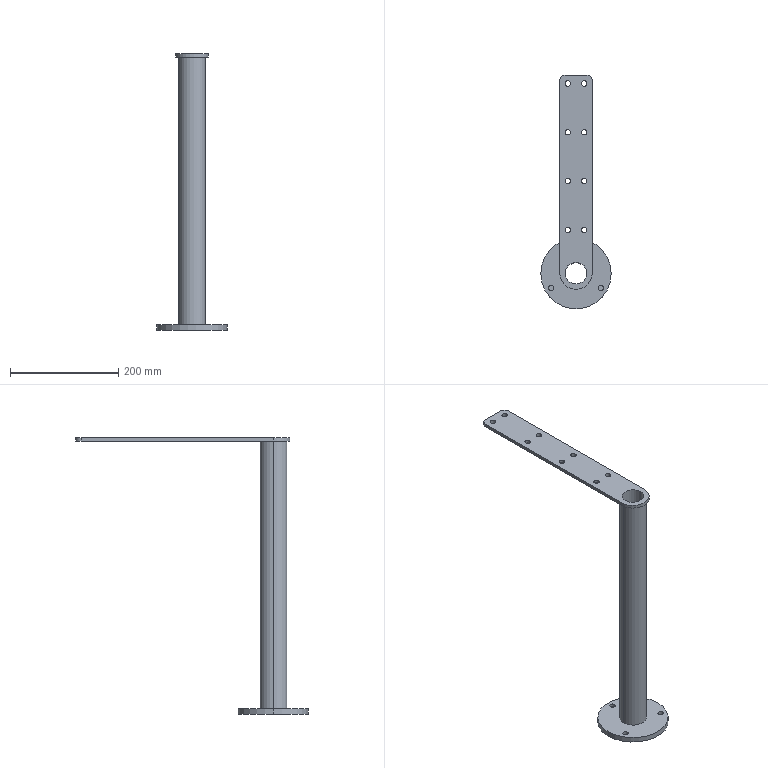Part | SolidWorks | features ICE 4, Extrusion 1, Fillet 1 | 1 solid | 41 faces | box 130 x 430 x 510 mm | volume 596255 mm3 | cylinder 31 | plane 10 | commonest cylinder face diameters 10 x22 20 x2 40 x2 50 x2 130 x2 60 x1
STEP:
#1=CARTESIAN_POINT('',(-5.,53.,4.));
#2=VERTEX_POINT('',#1);
#3=CARTESIAN_POINT('',(5.,53.,4.));
#4=VERTEX_POINT('',#3);
#5=CARTESIAN_POINT('',(0.,53.,4.));
#6=DIRECTION('',(0.,0.,1.));
#7=DIRECTION('',(1.,0.,0.));
#8=AXIS2_PLACEMENT_3D('',#5,#6,#7);
#9=CIRCLE('',#8,5.);
#10=EDGE_CURVE('',#2,#4,#9,.T.);
#11=ORIENTED_EDGE('',*,*,#10,.F.);
#12=CARTESIAN_POINT('',(-5.,53.,10.));
#13=VERTEX_POINT('',#12);
#14=CARTESIAN_POINT('',(-5.,53.,4.));
#15=DIRECTION('',(0.,0.,1.));
#16=VECTOR('',#15,1000.);
#17=LINE('',#14,#16);
#18=EDGE_CURVE('',#2,#13,#17,.T.);
#19=ORIENTED_EDGE('',*,*,#18,.T.);
#20=CARTESIAN_POINT('',(5.,53.,10.));
#21=VERTEX_POINT('',#20);
#22=CARTESIAN_POINT('',(0.,53.,10.));
#23=DIRECTION('',(0.,0.,1.));
#24=DIRECTION('',(1.,0.,0.));
#25=AXIS2_PLACEMENT_3D('',#22,#23,#24);
#26=CIRCLE('',#25,5.);
#27=EDGE_CURVE('',#13,#21,#26,.T.);
#28=ORIENTED_EDGE('',*,*,#27,.T.);
#29=CARTESIAN_POINT('',(5.,53.,4.));
#30=DIRECTION('',(0.,0.,1.));
#31=VECTOR('',#30,1000.);
#32=LINE('',#29,#31);
#33=EDGE_CURVE('',#4,#21,#32,.T.);
#34=ORIENTED_EDGE('',*,*,#33,.F.);
#35=EDGE_LOOP('',(#11,#19,#28,#34));
#36=FACE_OUTER_BOUND('',#35,.T.);
#37=CARTESIAN_POINT('',(0.,53.,4.));
#38=DIRECTION('',(0.,0.,1.));
#39=DIRECTION('',(1.,0.,0.));
#40=AXIS2_PLACEMENT_3D('',#37,#38,#39);
#41=CYLINDRICAL_SURFACE('',#40,5.);
#42=ADVANCED_FACE('',(#36),#41,.F.);
#43=CARTESIAN_POINT('',(40.899,-26.5,4.));
#44=VERTEX_POINT('',#43);
#45=CARTESIAN_POINT('',(50.899,-26.5,4.));
#46=VERTEX_POINT('',#45);
#47=CARTESIAN_POINT('',(45.899,-26.5,4.));
#48=DIRECTION('',(0.,0.,1.));
#49=DIRECTION('',(1.,0.,0.));
#50=AXIS2_PLACEMENT_3D('',#47,#48,#49);
#51=CIRCLE('',#50,5.);
#52=EDGE_CURVE('',#44,#46,#51,.T.);
#53=ORIENTED_EDGE('',*,*,#52,.F.);
#54=CARTESIAN_POINT('',(40.899,-26.5,10.));
#55=VERTEX_POINT('',#54);
#56=CARTESIAN_POINT('',(40.899,-26.5,4.));
#57=DIRECTION('',(0.,0.,1.));
#58=VECTOR('',#57,1000.);
#59=LINE('',#56,#58);
#60=EDGE_CURVE('',#44,#55,#59,.T.);
#61=ORIENTED_EDGE('',*,*,#60,.T.);
#62=CARTESIAN_POINT('',(50.899,-26.5,10.));
#63=VERTEX_POINT('',#62);
#64=CARTESIAN_POINT('',(45.899,-26.5,10.));
#65=DIRECTION('',(0.,0.,1.));
#66=DIRECTION('',(1.,0.,0.));
#67=AXIS2_PLACEMENT_3D('',#64,#65,#66);
#68=CIRCLE('',#67,5.);
#69=EDGE_CURVE('',#55,#63,#68,.T.);
#70=ORIENTED_EDGE('',*,*,#69,.T.);
#71=CARTESIAN_POINT('',(50.899,-26.5,4.));
#72=DIRECTION('',(0.,0.,1.));
#73=VECTOR('',#72,1000.);
#74=LINE('',#71,#73);
#75=EDGE_CURVE('',#46,#63,#74,.T.);
#76=ORIENTED_EDGE('',*,*,#75,.F.);
#77=EDGE_LOOP('',(#53,#61,#70,#76));
#78=FACE_OUTER_BOUND('',#77,.T.);
#79=CARTESIAN_POINT('',(45.899,-26.5,4.));
#80=DIRECTION('',(0.,0.,1.));
#81=DIRECTION('',(1.,0.,0.));
#82=AXIS2_PLACEMENT_3D('',#79,#80,#81);
#83=CYLINDRICAL_SURFACE('',#82,5.);
#84=ADVANCED_FACE('',(#78),#83,.F.);
#85=CARTESIAN_POINT('',(-50.899,-26.5,4.));
#86=VERTEX_POINT('',#85);
#87=CARTESIAN_POINT('',(-40.899,-26.5,4.));
#88=VERTEX_POINT('',#87);
#89=CARTESIAN_POINT('',(-45.899,-26.5,4.));
#90=DIRECTION('',(0.,0.,1.));
#91=DIRECTION('',(1.,0.,0.));
#92=AXIS2_PLACEMENT_3D('',#89,#90,#91);
#93=CIRCLE('',#92,5.);
#94=EDGE_CURVE('',#86,#88,#93,.T.);
#95=ORIENTED_EDGE('',*,*,#94,.F.);
#96=CARTESIAN_POINT('',(-50.899,-26.5,10.));
#97=VERTEX_POINT('',#96);
#98=CARTESIAN_POINT('',(-50.899,-26.5,4.));
#99=DIRECTION('',(0.,0.,1.));
#100=VECTOR('',#99,1000.);
#101=LINE('',#98,#100);
#102=EDGE_CURVE('',#86,#97,#101,.T.);
#103=ORIENTED_EDGE('',*,*,#102,.T.);
#104=CARTESIAN_POINT('',(-40.899,-26.5,10.));
#105=VERTEX_POINT('',#104);
#106=CARTESIAN_POINT('',(-45.899,-26.5,10.));
#107=DIRECTION('',(0.,0.,1.));
#108=DIRECTION('',(1.,0.,0.));
#109=AXIS2_PLACEMENT_3D('',#106,#107,#108);
#110=CIRCLE('',#109,5.);
#111=EDGE_CURVE('',#97,#105,#110,.T.);
#112=ORIENTED_EDGE('',*,*,#111,.T.);
#113=CARTESIAN_POINT('',(-40.899,-26.5,4.));
#114=DIRECTION('',(0.,0.,1.));
#115=VECTOR('',#114,1000.);
#116=LINE('',#113,#115);
#117=EDGE_CURVE('',#88,#105,#116,.T.);
#118=ORIENTED_EDGE('',*,*,#117,.F.);
#119=EDGE_LOOP('',(#95,#103,#112,#118));
#120=FACE_OUTER_BOUND('',#119,.T.);
#121=CARTESIAN_POINT('',(-45.899,-26.5,4.));
#122=DIRECTION('',(0.,0.,1.));
#123=DIRECTION('',(1.,0.,0.));
#124=AXIS2_PLACEMENT_3D('',#121,#122,#123);
#125=CYLINDRICAL_SURFACE('',#124,5.);
#126=ADVANCED_FACE('',(#120),#125,.F.);
#127=CARTESIAN_POINT('',(-20.,170.,504.));
#128=VERTEX_POINT('',#127);
#129=CARTESIAN_POINT('',(-10.,170.,504.));
#130=VERTEX_POINT('',#129);
#131=CARTESIAN_POINT('',(-15.,170.,504.));
#132=DIRECTION('',(0.,0.,1.));
#133=DIRECTION('',(1.,0.,0.));
#134=AXIS2_PLACEMENT_3D('',#131,#132,#133);
#135=CIRCLE('',#134,5.);
#136=EDGE_CURVE('',#128,#130,#135,.T.);
#137=ORIENTED_EDGE('',*,*,#136,.F.);
#138=CARTESIAN_POINT('',(-20.,170.,510.));
#139=VERTEX_POINT('',#138);
#140=CARTESIAN_POINT('',(-20.,170.,504.));
#141=DIRECTION('',(0.,0.,1.));
#142=VECTOR('',#141,1000.);
#143=LINE('',#140,#142);
#144=EDGE_CURVE('',#128,#139,#143,.T.);
#145=ORIENTED_EDGE('',*,*,#144,.T.);
#146=CARTESIAN_POINT('',(-10.,170.,510.));
#147=VERTEX_POINT('',#146);
#148=CARTESIAN_POINT('',(-15.,170.,510.));
#149=DIRECTION('',(0.,0.,1.));
#150=DIRECTION('',(1.,0.,0.));
#151=AXIS2_PLACEMENT_3D('',#148,#149,#150);
#152=CIRCLE('',#151,5.);
#153=EDGE_CURVE('',#139,#147,#152,.T.);
#154=ORIENTED_EDGE('',*,*,#153,.T.);
#155=CARTESIAN_POINT('',(-10.,170.,504.));
#156=DIRECTION('',(0.,0.,1.));
#157=VECTOR('',#156,1000.);
#158=LINE('',#155,#157);
#159=EDGE_CURVE('',#130,#147,#158,.T.);
#160=ORIENTED_EDGE('',*,*,#159,.F.);
#161=EDGE_LOOP('',(#137,#145,#154,#160));
#162=FACE_OUTER_BOUND('',#161,.T.);
#163=CARTESIAN_POINT('',(-15.,170.,504.));
#164=DIRECTION('',(0.,0.,1.));
#165=DIRECTION('',(1.,0.,0.));
#166=AXIS2_PLACEMENT_3D('',#163,#164,#165);
#167=CYLINDRICAL_SURFACE('',#166,5.);
#168=ADVANCED_FACE('',(#162),#167,.F.);
#169=CARTESIAN_POINT('',(10.,260.,504.));
#170=VERTEX_POINT('',#169);
#171=CARTESIAN_POINT('',(20.,260.,504.));
#172=VERTEX_POINT('',#171);
#173=CARTESIAN_POINT('',(15.,260.,504.));
#174=DIRECTION('',(0.,0.,1.));
#175=DIRECTION('',(1.,0.,0.));
#176=AXIS2_PLACEMENT_3D('',#173,#174,#175);
#177=CIRCLE('',#176,5.);
#178=EDGE_CURVE('',#170,#172,#177,.T.);
#179=ORIENTED_EDGE('',*,*,#178,.F.);
#180=CARTESIAN_POINT('',(10.,260.,510.));
#181=VERTEX_POINT('',#180);
#182=CARTESIAN_POINT('',(10.,260.,504.));
#183=DIRECTION('',(0.,0.,1.));
#184=VECTOR('',#183,1000.);
#185=LINE('',#182,#184);
#186=EDGE_CURVE('',#170,#181,#185,.T.);
#187=ORIENTED_EDGE('',*,*,#186,.T.);
#188=CARTESIAN_POINT('',(20.,260.,510.));
#189=VERTEX_POINT('',#188);
#190=CARTESIAN_POINT('',(15.,260.,510.));
#191=DIRECTION('',(0.,0.,1.));
#192=DIRECTION('',(1.,0.,0.));
#193=AXIS2_PLACEMENT_3D('',#190,#191,#192);
#194=CIRCLE('',#193,5.);
#195=EDGE_CURVE('',#181,#189,#194,.T.);
#196=ORIENTED_EDGE('',*,*,#195,.T.);
#197=CARTESIAN_POINT('',(20.,260.,504.));
#198=DIRECTION('',(0.,0.,1.));
#199=VECTOR('',#198,1000.);
#200=LINE('',#197,#199);
#201=EDGE_CURVE('',#172,#189,#200,.T.);
#202=ORIENTED_EDGE('',*,*,#201,.F.);
#203=EDGE_LOOP('',(#179,#187,#196,#202));
#204=FACE_OUTER_BOUND('',#203,.T.);
#205=CARTESIAN_POINT('',(15.,260.,504.));
#206=DIRECTION('',(0.,0.,1.));
#207=DIRECTION('',(1.,0.,0.));
#208=AXIS2_PLACEMENT_3D('',#205,#206,#207);
#209=CYLINDRICAL_SURFACE('',#208,5.);
#210=ADVANCED_FACE('',(#204),#209,.F.);
#211=CARTESIAN_POINT('',(-20.,260.,504.));
#212=VERTEX_POINT('',#211);
#213=CARTESIAN_POINT('',(-10.,260.,504.));
#214=VERTEX_POINT('',#213);
#215=CARTESIAN_POINT('',(-15.,260.,504.));
#216=DIRECTION('',(0.,0.,1.));
#217=DIRECTION('',(1.,0.,0.));
#218=AXIS2_PLACEMENT_3D('',#215,#216,#217);
#219=CIRCLE('',#218,5.);
#220=EDGE_CURVE('',#212,#214,#219,.T.);
#221=ORIENTED_EDGE('',*,*,#220,.F.);
#222=CARTESIAN_POINT('',(-20.,260.,510.));
#223=VERTEX_POINT('',#222);
#224=CARTESIAN_POINT('',(-20.,260.,504.));
#225=DIRECTION('',(0.,0.,1.));
#226=VECTOR('',#225,1000.);
#227=LINE('',#224,#226);
#228=EDGE_CURVE('',#212,#223,#227,.T.);
#229=ORIENTED_EDGE('',*,*,#228,.T.);
#230=CARTESIAN_POINT('',(-10.,260.,510.));
#231=VERTEX_POINT('',#230);
#232=CARTESIAN_POINT('',(-15.,260.,510.));
#233=DIRECTION('',(0.,0.,1.));
#234=DIRECTION('',(1.,0.,0.));
#235=AXIS2_PLACEMENT_3D('',#232,#233,#234);
#236=CIRCLE('',#235,5.);
#237=EDGE_CURVE('',#223,#231,#236,.T.);
#238=ORIENTED_EDGE('',*,*,#237,.T.);
#239=CARTESIAN_POINT('',(-10.,260.,504.));
#240=DIRECTION('',(0.,0.,1.));
#241=VECTOR('',#240,1000.);
#242=LINE('',#239,#241);
#243=EDGE_CURVE('',#214,#231,#242,.T.);
#244=ORIENTED_EDGE('',*,*,#243,.F.);
#245=EDGE_LOOP('',(#221,#229,#238,#244));
#246=FACE_OUTER_BOUND('',#245,.T.);
#247=CARTESIAN_POINT('',(-15.,260.,504.));
#248=DIRECTION('',(0.,0.,1.));
#249=DIRECTION('',(1.,0.,0.));
#250=AXIS2_PLACEMENT_3D('',#247,#248,#249);
#251=CYLINDRICAL_SURFACE('',#250,5.);
#252=ADVANCED_FACE('',(#246),#251,.F.);
#253=CARTESIAN_POINT('',(10.,350.,504.));
#254=VERTEX_POINT('',#253);
#255=CARTESIAN_POINT('',(20.,350.,504.));
#256=VERTEX_POINT('',#255);
#257=CARTESIAN_POINT('',(15.,350.,504.));
#258=DIRECTION('',(0.,0.,1.));
#259=DIRECTION('',(1.,0.,0.));
#260=AXIS2_PLACEMENT_3D('',#257,#258,#259);
#261=CIRCLE('',#260,5.);
#262=EDGE_CURVE('',#254,#256,#261,.T.);
#263=ORIENTED_EDGE('',*,*,#262,.F.);
#264=CARTESIAN_POINT('',(10.,350.,510.));
#265=VERTEX_POINT('',#264);
#266=CARTESIAN_POINT('',(10.,350.,504.));
#267=DIRECTION('',(0.,0.,1.));
#268=VECTOR('',#267,1000.);
#269=LINE('',#266,#268);
#270=EDGE_CURVE('',#254,#265,#269,.T.);
#271=ORIENTED_EDGE('',*,*,#270,.T.);
#272=CARTESIAN_POINT('',(20.,350.,510.));
#273=VERTEX_POINT('',#272);
#274=CARTESIAN_POINT('',(15.,350.,510.));
#275=DIRECTION('',(0.,0.,1.));
#276=DIRECTION('',(1.,0.,0.));
#277=AXIS2_PLACEMENT_3D('',#274,#275,#276);
#278=CIRCLE('',#277,5.);
#279=EDGE_CURVE('',#265,#273,#278,.T.);
#280=ORIENTED_EDGE('',*,*,#279,.T.);
#281=CARTESIAN_POINT('',(20.,350.,504.));
#282=DIRECTION('',(0.,0.,1.));
#283=VECTOR('',#282,1000.);
#284=LINE('',#281,#283);
#285=EDGE_CURVE('',#256,#273,#284,.T.);
#286=ORIENTED_EDGE('',*,*,#285,.F.);
#287=EDGE_LOOP('',(#263,#271,#280,#286));
#288=FACE_OUTER_BOUND('',#287,.T.);
#289=CARTESIAN_POINT('',(15.,350.,504.));
#290=DIRECTION('',(0.,0.,1.));
#291=DIRECTION('',(1.,0.,0.));
#292=AXIS2_PLACEMENT_3D('',#289,#290,#291);
#293=CYLINDRICAL_SURFACE('',#292,5.);
#294=ADVANCED_FACE('',(#288),#293,.F.);
#295=CARTESIAN_POINT('',(10.,80.,504.));
#296=VERTEX_POINT('',#295);
#297=CARTESIAN_POINT('',(20.,80.,504.));
#298=VERTEX_POINT('',#297);
#299=CARTESIAN_POINT('',(15.,80.,504.));
#300=DIRECTION('',(0.,0.,1.));
#301=DIRECTION('',(1.,0.,0.));
#302=AXIS2_PLACEMENT_3D('',#299,#300,#301);
#303=CIRCLE('',#302,5.);
#304=EDGE_CURVE('',#296,#298,#303,.T.);
#305=ORIENTED_EDGE('',*,*,#304,.F.);
#306=CARTESIAN_POINT('',(10.,80.,510.));
#307=VERTEX_POINT('',#306);
#308=CARTESIAN_POINT('',(10.,80.,504.));
#309=DIRECTION('',(0.,0.,1.));
#310=VECTOR('',#309,1000.);
#311=LINE('',#308,#310);
#312=EDGE_CURVE('',#296,#307,#311,.T.);
#313=ORIENTED_EDGE('',*,*,#312,.T.);
#314=CARTESIAN_POINT('',(20.,80.,510.));
#315=VERTEX_POINT('',#314);
#316=CARTESIAN_POINT('',(15.,80.,510.));
#317=DIRECTION('',(0.,0.,1.));
#318=DIRECTION('',(1.,0.,0.));
#319=AXIS2_PLACEMENT_3D('',#316,#317,#318);
#320=CIRCLE('',#319,5.);
#321=EDGE_CURVE('',#307,#315,#320,.T.);
#322=ORIENTED_EDGE('',*,*,#321,.T.);
#323=CARTESIAN_POINT('',(20.,80.,504.));
#324=DIRECTION('',(0.,0.,1.));
#325=VECTOR('',#324,1000.);
#326=LINE('',#323,#325);
#327=EDGE_CURVE('',#298,#315,#326,.T.);
#328=ORIENTED_EDGE('',*,*,#327,.F.);
#329=EDGE_LOOP('',(#305,#313,#322,#328));
#330=FACE_OUTER_BOUND('',#329,.T.);
#331=CARTESIAN_POINT('',(15.,80.,504.));
#332=DIRECTION('',(0.,0.,1.));
#333=DIRECTION('',(1.,0.,0.));
#334=AXIS2_PLACEMENT_3D('',#331,#332,#333);
#335=CYLINDRICAL_SURFACE('',#334,5.);
#336=ADVANCED_FACE('',(#330),#335,.F.);
#337=CARTESIAN_POINT('',(-20.,80.,504.));
#338=VERTEX_POINT('',#337);
#339=CARTESIAN_POINT('',(-10.,80.,504.));
#340=VERTEX_POINT('',#339);
#341=CARTESIAN_POINT('',(-15.,80.,504.));
#342=DIRECTION('',(0.,0.,1.));
#343=DIRECTION('',(1.,0.,0.));
#344=AXIS2_PLACEMENT_3D('',#341,#342,#343);
#345=CIRCLE('',#344,5.);
#346=EDGE_CURVE('',#338,#340,#345,.T.);
#347=ORIENTED_EDGE('',*,*,#346,.F.);
#348=CARTESIAN_POINT('',(-20.,80.,510.));
#349=VERTEX_POINT('',#348);
#350=CARTESIAN_POINT('',(-20.,80.,504.));
#351=DIRECTION('',(0.,0.,1.));
#352=VECTOR('',#351,1000.);
#353=LINE('',#350,#352);
#354=EDGE_CURVE('',#338,#349,#353,.T.);
#355=ORIENTED_EDGE('',*,*,#354,.T.);
#356=CARTESIAN_POINT('',(-10.,80.,510.));
#357=VERTEX_POINT('',#356);
#358=CARTESIAN_POINT('',(-15.,80.,510.));
#359=DIRECTION('',(0.,0.,1.));
#360=DIRECTION('',(1.,0.,0.));
#361=AXIS2_PLACEMENT_3D('',#358,#359,#360);
#362=CIRCLE('',#361,5.);
#363=EDGE_CURVE('',#349,#357,#362,.T.);
#364=ORIENTED_EDGE('',*,*,#363,.T.);
#365=CARTESIAN_POINT('',(-10.,80.,504.));
#366=DIRECTION('',(0.,0.,1.));
#367=VECTOR('',#366,1000.);
#368=LINE('',#365,#367);
#369=EDGE_CURVE('',#340,#357,#368,.T.);
#370=ORIENTED_EDGE('',*,*,#369,.F.);
#371=EDGE_LOOP('',(#347,#355,#364,#370));
#372=FACE_OUTER_BOUND('',#371,.T.);
#373=CARTESIAN_POINT('',(-15.,80.,504.));
#374=DIRECTION('',(0.,0.,1.));
#375=DIRECTION('',(1.,0.,0.));
#376=AXIS2_PLACEMENT_3D('',#373,#374,#375);
#377=CYLINDRICAL_SURFACE('',#376,5.);
#378=ADVANCED_FACE('',(#372),#377,.F.);
#379=CARTESIAN_POINT('',(10.,170.,504.));
#380=VERTEX_POINT('',#379);
#381=CARTESIAN_POINT('',(20.,170.,504.));
#382=VERTEX_POINT('',#381);
#383=CARTESIAN_POINT('',(15.,170.,504.));
#384=DIRECTION('',(0.,0.,1.));
#385=DIRECTION('',(1.,0.,0.));
#386=AXIS2_PLACEMENT_3D('',#383,#384,#385);
#387=CIRCLE('',#386,5.);
#388=EDGE_CURVE('',#380,#382,#387,.T.);
#389=ORIENTED_EDGE('',*,*,#388,.F.);
#390=CARTESIAN_POINT('',(10.,170.,510.));
#391=VERTEX_POINT('',#390);
#392=CARTESIAN_POINT('',(10.,170.,504.));
#393=DIRECTION('',(0.,0.,1.));
#394=VECTOR('',#393,1000.);
#395=LINE('',#392,#394);
#396=EDGE_CURVE('',#380,#391,#395,.T.);
#397=ORIENTED_EDGE('',*,*,#396,.T.);
#398=CARTESIAN_POINT('',(20.,170.,510.));
#399=VERTEX_POINT('',#398);
#400=CARTESIAN_POINT('',(15.,170.,510.));
#401=DIRECTION('',(0.,0.,1.));
#402=DIRECTION('',(1.,0.,0.));
#403=AXIS2_PLACEMENT_3D('',#400,#401,#402);
#404=CIRCLE('',#403,5.);
#405=EDGE_CURVE('',#391,#399,#404,.T.);
#406=ORIENTED_EDGE('',*,*,#405,.T.);
#407=CARTESIAN_POINT('',(20.,170.,504.));
#408=DIRECTION('',(0.,0.,1.));
#409=VECTOR('',#408,1000.);
#410=LINE('',#407,#409);
#411=EDGE_CURVE('',#382,#399,#410,.T.);
#412=ORIENTED_EDGE('',*,*,#411,.F.);
#413=EDGE_LOOP('',(#389,#397,#406,#412));
#414=FACE_OUTER_BOUND('',#413,.T.);
#415=CARTESIAN_POINT('',(15.,170.,504.));
#416=DIRECTION('',(0.,0.,1.));
#417=DIRECTION('',(1.,0.,0.));
#418=AXIS2_PLACEMENT_3D('',#415,#416,#417);
#419=CYLINDRICAL_SURFACE('',#418,5.);
#420=ADVANCED_FACE('',(#414),#419,.F.);
#421=CARTESIAN_POINT('',(-20.,350.,504.));
#422=VERTEX_POINT('',#421);
#423=CARTESIAN_POINT('',(-10.,350.,504.));
#424=VERTEX_POINT('',#423);
#425=CARTESIAN_POINT('',(-15.,350.,504.));
#426=DIRECTION('',(0.,0.,1.));
#427=DIRECTION('',(1.,0.,0.));
#428=AXIS2_PLACEMENT_3D('',#425,#426,#427);
#429=CIRCLE('',#428,5.);
#430=EDGE_CURVE('',#422,#424,#429,.T.);
#431=ORIENTED_EDGE('',*,*,#430,.F.);
#432=CARTESIAN_POINT('',(-20.,350.,510.));
#433=VERTEX_POINT('',#432);
#434=CARTESIAN_POINT('',(-20.,350.,504.));
#435=DIRECTION('',(0.,0.,1.));
#436=VECTOR('',#435,1000.);
#437=LINE('',#434,#436);
#438=EDGE_CURVE('',#422,#433,#437,.T.);
#439=ORIENTED_EDGE('',*,*,#438,.T.);
#440=CARTESIAN_POINT('',(-10.,350.,510.));
#441=VERTEX_POINT('',#440);
#442=CARTESIAN_POINT('',(-15.,350.,510.));
#443=DIRECTION('',(0.,0.,1.));
#444=DIRECTION('',(1.,0.,0.));
#445=AXIS2_PLACEMENT_3D('',#442,#443,#444);
#446=CIRCLE('',#445,5.);
#447=EDGE_CURVE('',#433,#441,#446,.T.);
#448=ORIENTED_EDGE('',*,*,#447,.T.);
#449=CARTESIAN_POINT('',(-10.,350.,504.));
#450=DIRECTION('',(0.,0.,1.));
#451=VECTOR('',#450,1000.);
#452=LINE('',#449,#451);
#453=EDGE_CURVE('',#424,#441,#452,.T.);
#454=ORIENTED_EDGE('',*,*,#453,.F.);
#455=EDGE_LOOP('',(#431,#439,#448,#454));
#456=FACE_OUTER_BOUND('',#455,.T.);
#457=CARTESIAN_POINT('',(-15.,350.,504.));
#458=DIRECTION('',(0.,0.,1.));
#459=DIRECTION('',(1.,0.,0.));
#460=AXIS2_PLACEMENT_3D('',#457,#458,#459);
#461=CYLINDRICAL_SURFACE('',#460,5.);
#462=ADVANCED_FACE('',(#456),#461,.F.);
#463=CARTESIAN_POINT('',(25.,0.,504.));
#464=VERTEX_POINT('',#463);
#465=CARTESIAN_POINT('',(-25.,0.,504.));
#466=VERTEX_POINT('',#465);
#467=CARTESIAN_POINT('',(0.,0.,504.));
#468=DIRECTION('',(0.,0.,1.));
#469=DIRECTION('',(1.,0.,0.));
#470=AXIS2_PLACEMENT_3D('',#467,#468,#469);
#471=CIRCLE('',#470,25.);
#472=EDGE_CURVE('',#464,#466,#471,.T.);
#473=ORIENTED_EDGE('',*,*,#472,.F.);
#474=CARTESIAN_POINT('',(25.,0.,10.));
#475=VERTEX_POINT('',#474);
#476=CARTESIAN_POINT('',(25.,0.,504.));
#477=DIRECTION('',(0.,0.,-1.));
#478=VECTOR('',#477,1000.);
#479=LINE('',#476,#478);
#480=EDGE_CURVE('',#464,#475,#479,.T.);
#481=ORIENTED_EDGE('',*,*,#480,.T.);
#482=CARTESIAN_POINT('',(-25.,0.,10.));
#483=VERTEX_POINT('',#482);
#484=CARTESIAN_POINT('',(0.,0.,10.));
#485=DIRECTION('',(0.,0.,1.));
#486=DIRECTION('',(1.,0.,0.));
#487=AXIS2_PLACEMENT_3D('',#484,#485,#486);
#488=CIRCLE('',#487,25.);
#489=EDGE_CURVE('',#475,#483,#488,.T.);
#490=ORIENTED_EDGE('',*,*,#489,.T.);
#491=CARTESIAN_POINT('',(-25.,0.,504.));
#492=DIRECTION('',(0.,0.,-1.));
#493=VECTOR('',#492,1000.);
#494=LINE('',#491,#493);
#495=EDGE_CURVE('',#466,#483,#494,.T.);
#496=ORIENTED_EDGE('',*,*,#495,.F.);
#497=EDGE_LOOP('',(#473,#481,#490,#496));
#498=FACE_OUTER_BOUND('',#497,.T.);
#499=CARTESIAN_POINT('',(0.,0.,504.));
#500=DIRECTION('',(0.,0.,-1.));
#501=DIRECTION('',(-1.,0.,0.));
#502=AXIS2_PLACEMENT_3D('',#499,#500,#501);
#503=CYLINDRICAL_SURFACE('',#502,25.);
#504=ADVANCED_FACE('',(#498),#503,.T.);
#505=CARTESIAN_POINT('',(-20.,0.,510.));
#506=VERTEX_POINT('',#505);
#507=CARTESIAN_POINT('',(20.,0.,510.));
#508=VERTEX_POINT('',#507);
#509=CARTESIAN_POINT('',(0.,0.,510.));
#510=DIRECTION('',(0.,0.,1.));
#511=DIRECTION('',(1.,0.,0.));
#512=AXIS2_PLACEMENT_3D('',#509,#510,#511);
#513=CIRCLE('',#512,20.);
#514=EDGE_CURVE('',#506,#508,#513,.T.);
#515=ORIENTED_EDGE('',*,*,#514,.T.);
#516=CARTESIAN_POINT('',(20.,0.,0.));
#517=VERTEX_POINT('',#516);
#518=CARTESIAN_POINT('',(20.,0.,10.));
#519=DIRECTION('',(0.,0.,-1.));
#520=VECTOR('',#519,1000.);
#521=LINE('',#518,#520);
#522=EDGE_CURVE('',#508,#517,#521,.T.);
#523=ORIENTED_EDGE('',*,*,#522,.T.);
#524=CARTESIAN_POINT('',(-20.,0.,0.));
#525=VERTEX_POINT('',#524);
#526=CARTESIAN_POINT('',(0.,0.,0.));
#527=DIRECTION('',(0.,0.,1.));
#528=DIRECTION('',(1.,0.,0.));
#529=AXIS2_PLACEMENT_3D('',#526,#527,#528);
#530=CIRCLE('',#529,20.);
#531=EDGE_CURVE('',#525,#517,#530,.T.);
#532=ORIENTED_EDGE('',*,*,#531,.F.);
#533=CARTESIAN_POINT('',(-20.,0.,10.));
#534=DIRECTION('',(0.,0.,-1.));
#535=VECTOR('',#534,1000.);
#536=LINE('',#533,#535);
#537=EDGE_CURVE('',#506,#525,#536,.T.);
#538=ORIENTED_EDGE('',*,*,#537,.F.);
#539=EDGE_LOOP('',(#515,#523,#532,#538));
#540=FACE_OUTER_BOUND('',#539,.T.);
#541=CARTESIAN_POINT('',(0.,0.,10.));
#542=DIRECTION('',(0.,0.,-1.));
#543=DIRECTION('',(-1.,0.,0.));
#544=AXIS2_PLACEMENT_3D('',#541,#542,#543);
#545=CYLINDRICAL_SURFACE('',#544,20.);
#546=ADVANCED_FACE('',(#540),#545,.F.);
#547=CARTESIAN_POINT('',(65.,0.,10.));
#548=VERTEX_POINT('',#547);
#549=CARTESIAN_POINT('',(-65.,0.,10.));
#550=VERTEX_POINT('',#549);
#551=CARTESIAN_POINT('',(0.,0.,10.));
#552=DIRECTION('',(0.,0.,1.));
#553=DIRECTION('',(1.,0.,0.));
#554=AXIS2_PLACEMENT_3D('',#551,#552,#553);
#555=CIRCLE('',#554,65.);
#556=EDGE_CURVE('',#548,#550,#555,.T.);
#557=ORIENTED_EDGE('',*,*,#556,.F.);
#558=CARTESIAN_POINT('',(65.,0.,0.));
#559=VERTEX_POINT('',#558);
#560=CARTESIAN_POINT('',(65.,0.,10.));
#561=DIRECTION('',(0.,0.,-1.));
#562=VECTOR('',#561,1000.);
#563=LINE('',#560,#562);
#564=EDGE_CURVE('',#548,#559,#563,.T.);
#565=ORIENTED_EDGE('',*,*,#564,.T.);
#566=CARTESIAN_POINT('',(-65.,0.,0.));
#567=VERTEX_POINT('',#566);
#568=CARTESIAN_POINT('',(0.,0.,0.));
#569=DIRECTION('',(0.,0.,1.));
#570=DIRECTION('',(1.,0.,0.));
#571=AXIS2_PLACEMENT_3D('',#568,#569,#570);
#572=CIRCLE('',#571,65.);
#573=EDGE_CURVE('',#559,#567,#572,.T.);
#574=ORIENTED_EDGE('',*,*,#573,.T.);
#575=CARTESIAN_POINT('',(-65.,0.,10.));
#576=DIRECTION('',(0.,0.,-1.));
#577=VECTOR('',#576,1000.);
#578=LINE('',#575,#577);
#579=EDGE_CURVE('',#550,#567,#578,.T.);
#580=ORIENTED_EDGE('',*,*,#579,.F.);
#581=EDGE_LOOP('',(#557,#565,#574,#580));
#582=FACE_OUTER_BOUND('',#581,.T.);
#583=CARTESIAN_POINT('',(0.,0.,10.));
#584=DIRECTION('',(0.,0.,-1.));
#585=DIRECTION('',(-1.,0.,0.));
#586=AXIS2_PLACEMENT_3D('',#583,#584,#585);
#587=CYLINDRICAL_SURFACE('',#586,65.);
#588=ADVANCED_FACE('',(#582),#587,.T.);
#589=CARTESIAN_POINT('',(0.,53.,10.));
#590=DIRECTION('',(0.,0.,1.));
#591=DIRECTION('',(1.,0.,0.));
#592=AXIS2_PLACEMENT_3D('',#589,#590,#591);
#593=CIRCLE('',#592,5.);
#594=EDGE_CURVE('',#21,#13,#593,.T.);
#595=ORIENTED_EDGE('',*,*,#594,.F.);
#596=ORIENTED_EDGE('',*,*,#27,.F.);
#597=EDGE_LOOP('',(#595,#596));
#598=FACE_BOUND('',#597,.T.);
#599=CARTESIAN_POINT('',(45.899,-26.5,10.));
#600=DIRECTION('',(0.,0.,1.));
#601=DIRECTION('',(1.,0.,0.));
#602=AXIS2_PLACEMENT_3D('',#599,#600,#601);
#603=CIRCLE('',#602,5.);
#604=EDGE_CURVE('',#63,#55,#603,.T.);
#605=ORIENTED_EDGE('',*,*,#604,.F.);
#606=ORIENTED_EDGE('',*,*,#69,.F.);
#607=EDGE_LOOP('',(#605,#606));
#608=FACE_BOUND('',#607,.T.);
#609=CARTESIAN_POINT('',(-45.899,-26.5,10.));
#610=DIRECTION('',(0.,0.,1.));
#611=DIRECTION('',(1.,0.,0.));
#612=AXIS2_PLACEMENT_3D('',#609,#610,#611);
#613=CIRCLE('',#612,5.);
#614=EDGE_CURVE('',#105,#97,#613,.T.);
#615=ORIENTED_EDGE('',*,*,#614,.F.);
#616=ORIENTED_EDGE('',*,*,#111,.F.);
#617=EDGE_LOOP('',(#615,#616));
#618=FACE_BOUND('',#617,.T.);
#619=CARTESIAN_POINT('',(0.,0.,10.));
#620=DIRECTION('',(0.,0.,1.));
#621=DIRECTION('',(1.,0.,0.));
#622=AXIS2_PLACEMENT_3D('',#619,#620,#621);
#623=CIRCLE('',#622,65.);
#624=EDGE_CURVE('',#550,#548,#623,.T.);
#625=ORIENTED_EDGE('',*,*,#624,.T.);
#626=ORIENTED_EDGE('',*,*,#556,.T.);
#627=EDGE_LOOP('',(#625,#626));
#628=FACE_OUTER_BOUND('',#627,.T.);
#629=CARTESIAN_POINT('',(0.,0.,10.));
#630=DIRECTION('',(0.,0.,1.));
#631=DIRECTION('',(1.,0.,0.));
#632=AXIS2_PLACEMENT_3D('',#629,#630,#631);
#633=CIRCLE('',#632,25.);
#634=EDGE_CURVE('',#483,#475,#633,.T.);
#635=ORIENTED_EDGE('',*,*,#634,.F.);
#636=ORIENTED_EDGE('',*,*,#489,.F.);
#637=EDGE_LOOP('',(#635,#636));
#638=FACE_BOUND('',#637,.T.);
#639=CARTESIAN_POINT('',(0.,0.,10.));
#640=DIRECTION('',(0.,0.,1.));
#641=DIRECTION('',(1.,0.,0.));
#642=AXIS2_PLACEMENT_3D('',#639,#640,#641);
#643=PLANE('',#642);
#644=ADVANCED_FACE('',(#598,#608,#618,#628,#638),#643,.T.);
#645=CARTESIAN_POINT('',(0.,0.,0.));
#646=DIRECTION('',(0.,0.,1.));
#647=DIRECTION('',(1.,0.,0.));
#648=AXIS2_PLACEMENT_3D('',#645,#646,#647);
#649=CIRCLE('',#648,65.);
#650=EDGE_CURVE('',#567,#559,#649,.T.);
#651=ORIENTED_EDGE('',*,*,#650,.F.);
#652=ORIENTED_EDGE('',*,*,#573,.F.);
#653=EDGE_LOOP('',(#651,#652));
#654=FACE_OUTER_BOUND('',#653,.T.);
#655=ORIENTED_EDGE('',*,*,#531,.T.);
#656=CARTESIAN_POINT('',(0.,0.,0.));
#657=DIRECTION('',(0.,0.,1.));
#658=DIRECTION('',(1.,0.,0.));
#659=AXIS2_PLACEMENT_3D('',#656,#657,#658);
#660=CIRCLE('',#659,20.);
#661=EDGE_CURVE('',#517,#525,#660,.T.);
#662=ORIENTED_EDGE('',*,*,#661,.T.);
#663=EDGE_LOOP('',(#655,#662));
#664=FACE_BOUND('',#663,.T.);
#665=CARTESIAN_POINT('',(0.,0.,0.));
#666=DIRECTION('',(0.,0.,1.));
#667=DIRECTION('',(1.,0.,0.));
#668=AXIS2_PLACEMENT_3D('',#665,#666,#667);
#669=PLANE('',#668);
#670=ADVANCED_FACE('',(#654,#664),#669,.F.);
#671=ORIENTED_EDGE('',*,*,#564,.F.);
#672=ORIENTED_EDGE('',*,*,#624,.F.);
#673=ORIENTED_EDGE('',*,*,#579,.T.);
#674=ORIENTED_EDGE('',*,*,#650,.T.);
#675=EDGE_LOOP('',(#671,#672,#673,#674));
#676=FACE_OUTER_BOUND('',#675,.T.);
#677=CARTESIAN_POINT('',(0.,0.,10.));
#678=DIRECTION('',(0.,0.,-1.));
#679=DIRECTION('',(-1.,0.,0.));
#680=AXIS2_PLACEMENT_3D('',#677,#678,#679);
#681=CYLINDRICAL_SURFACE('',#680,65.);
#682=ADVANCED_FACE('',(#676),#681,.T.);
#683=ORIENTED_EDGE('',*,*,#522,.F.);
#684=CARTESIAN_POINT('',(0.,0.,510.));
#685=DIRECTION('',(0.,0.,1.));
#686=DIRECTION('',(1.,0.,0.));
#687=AXIS2_PLACEMENT_3D('',#684,#685,#686);
#688=CIRCLE('',#687,20.);
#689=EDGE_CURVE('',#508,#506,#688,.T.);
#690=ORIENTED_EDGE('',*,*,#689,.T.);
#691=ORIENTED_EDGE('',*,*,#537,.T.);
#692=ORIENTED_EDGE('',*,*,#661,.F.);
#693=EDGE_LOOP('',(#683,#690,#691,#692));
#694=FACE_OUTER_BOUND('',#693,.T.);
#695=CARTESIAN_POINT('',(0.,0.,10.));
#696=DIRECTION('',(0.,0.,-1.));
#697=DIRECTION('',(-1.,0.,0.));
#698=AXIS2_PLACEMENT_3D('',#695,#696,#697);
#699=CYLINDRICAL_SURFACE('',#698,20.);
#700=ADVANCED_FACE('',(#694),#699,.F.);
#701=ORIENTED_EDGE('',*,*,#480,.F.);
#702=CARTESIAN_POINT('',(0.,0.,504.));
#703=DIRECTION('',(0.,0.,1.));
#704=DIRECTION('',(1.,0.,0.));
#705=AXIS2_PLACEMENT_3D('',#702,#703,#704);
#706=CIRCLE('',#705,25.);
#707=EDGE_CURVE('',#466,#464,#706,.T.);
#708=ORIENTED_EDGE('',*,*,#707,.F.);
#709=ORIENTED_EDGE('',*,*,#495,.T.);
#710=ORIENTED_EDGE('',*,*,#634,.T.);
#711=EDGE_LOOP('',(#701,#708,#709,#710));
#712=FACE_OUTER_BOUND('',#711,.T.);
#713=CARTESIAN_POINT('',(0.,0.,504.));
#714=DIRECTION('',(0.,0.,-1.));
#715=DIRECTION('',(-1.,0.,0.));
#716=AXIS2_PLACEMENT_3D('',#713,#714,#715);
#717=CYLINDRICAL_SURFACE('',#716,25.);
#718=ADVANCED_FACE('',(#712),#717,.T.);
#719=CARTESIAN_POINT('',(-15.,170.,510.));
#720=DIRECTION('',(0.,0.,1.));
#721=DIRECTION('',(1.,0.,0.));
#722=AXIS2_PLACEMENT_3D('',#719,#720,#721);
#723=CIRCLE('',#722,5.);
#724=EDGE_CURVE('',#147,#139,#723,.T.);
#725=ORIENTED_EDGE('',*,*,#724,.F.);
#726=ORIENTED_EDGE('',*,*,#153,.F.);
#727=EDGE_LOOP('',(#725,#726));
#728=FACE_BOUND('',#727,.T.);
#729=CARTESIAN_POINT('',(15.,260.,510.));
#730=DIRECTION('',(0.,0.,1.));
#731=DIRECTION('',(1.,0.,0.));
#732=AXIS2_PLACEMENT_3D('',#729,#730,#731);
#733=CIRCLE('',#732,5.);
#734=EDGE_CURVE('',#189,#181,#733,.T.);
#735=ORIENTED_EDGE('',*,*,#734,.F.);
#736=ORIENTED_EDGE('',*,*,#195,.F.);
#737=EDGE_LOOP('',(#735,#736));
#738=FACE_BOUND('',#737,.T.);
#739=CARTESIAN_POINT('',(-15.,260.,510.));
#740=DIRECTION('',(0.,0.,1.));
#741=DIRECTION('',(1.,0.,0.));
#742=AXIS2_PLACEMENT_3D('',#739,#740,#741);
#743=CIRCLE('',#742,5.);
#744=EDGE_CURVE('',#231,#223,#743,.T.);
#745=ORIENTED_EDGE('',*,*,#744,.F.);
#746=ORIENTED_EDGE('',*,*,#237,.F.);
#747=EDGE_LOOP('',(#745,#746));
#748=FACE_BOUND('',#747,.T.);
#749=CARTESIAN_POINT('',(15.,350.,510.));
#750=DIRECTION('',(0.,0.,1.));
#751=DIRECTION('',(1.,0.,0.));
#752=AXIS2_PLACEMENT_3D('',#749,#750,#751);
#753=CIRCLE('',#752,5.);
#754=EDGE_CURVE('',#273,#265,#753,.T.);
#755=ORIENTED_EDGE('',*,*,#754,.F.);
#756=ORIENTED_EDGE('',*,*,#279,.F.);
#757=EDGE_LOOP('',(#755,#756));
#758=FACE_BOUND('',#757,.T.);
#759=CARTESIAN_POINT('',(15.,80.,510.));
#760=DIRECTION('',(0.,0.,1.));
#761=DIRECTION('',(1.,0.,0.));
#762=AXIS2_PLACEMENT_3D('',#759,#760,#761);
#763=CIRCLE('',#762,5.);
#764=EDGE_CURVE('',#315,#307,#763,.T.);
#765=ORIENTED_EDGE('',*,*,#764,.F.);
#766=ORIENTED_EDGE('',*,*,#321,.F.);
#767=EDGE_LOOP('',(#765,#766));
#768=FACE_BOUND('',#767,.T.);
#769=CARTESIAN_POINT('',(-15.,80.,510.));
#770=DIRECTION('',(0.,0.,1.));
#771=DIRECTION('',(1.,0.,0.));
#772=AXIS2_PLACEMENT_3D('',#769,#770,#771);
#773=CIRCLE('',#772,5.);
#774=EDGE_CURVE('',#357,#349,#773,.T.);
#775=ORIENTED_EDGE('',*,*,#774,.F.);
#776=ORIENTED_EDGE('',*,*,#363,.F.);
#777=EDGE_LOOP('',(#775,#776));
#778=FACE_BOUND('',#777,.T.);
#779=CARTESIAN_POINT('',(15.,170.,510.));
#780=DIRECTION('',(0.,0.,1.));
#781=DIRECTION('',(1.,0.,0.));
#782=AXIS2_PLACEMENT_3D('',#779,#780,#781);
#783=CIRCLE('',#782,5.);
#784=EDGE_CURVE('',#399,#391,#783,.T.);
#785=ORIENTED_EDGE('',*,*,#784,.F.);
#786=ORIENTED_EDGE('',*,*,#405,.F.);
#787=EDGE_LOOP('',(#785,#786));
#788=FACE_BOUND('',#787,.T.);
#789=CARTESIAN_POINT('',(-15.,350.,510.));
#790=DIRECTION('',(0.,0.,1.));
#791=DIRECTION('',(1.,0.,0.));
#792=AXIS2_PLACEMENT_3D('',#789,#790,#791);
#793=CIRCLE('',#792,5.);
#794=EDGE_CURVE('',#441,#433,#793,.T.);
#795=ORIENTED_EDGE('',*,*,#794,.F.);
#796=ORIENTED_EDGE('',*,*,#447,.F.);
#797=EDGE_LOOP('',(#795,#796));
#798=FACE_BOUND('',#797,.T.);
#799=CARTESIAN_POINT('',(20.,365.,510.));
#800=VERTEX_POINT('',#799);
#801=CARTESIAN_POINT('',(-20.,365.,510.));
#802=VERTEX_POINT('',#801);
#803=CARTESIAN_POINT('',(-30.,365.,510.));
#804=DIRECTION('',(-1.,0.,0.));
#805=VECTOR('',#804,1000.);
#806=LINE('',#803,#805);
#807=EDGE_CURVE('',#800,#802,#806,.T.);
#808=ORIENTED_EDGE('',*,*,#807,.T.);
#809=CARTESIAN_POINT('',(-30.,355.,510.));
#810=VERTEX_POINT('',#809);
#811=CARTESIAN_POINT('',(-20.,355.,510.));
#812=DIRECTION('',(0.,0.,1.));
#813=DIRECTION('',(1.,0.,0.));
#814=AXIS2_PLACEMENT_3D('',#811,#812,#813);
#815=CIRCLE('',#814,10.);
#816=EDGE_CURVE('',#802,#810,#815,.T.);
#817=ORIENTED_EDGE('',*,*,#816,.T.);
#818=CARTESIAN_POINT('',(-30.,0.,510.));
#819=VERTEX_POINT('',#818);
#820=CARTESIAN_POINT('',(-30.,0.,510.));
#821=DIRECTION('',(0.,-1.,0.));
#822=VECTOR('',#821,1000.);
#823=LINE('',#820,#822);
#824=EDGE_CURVE('',#810,#819,#823,.T.);
#825=ORIENTED_EDGE('',*,*,#824,.T.);
#826=CARTESIAN_POINT('',(30.,0.,510.));
#827=VERTEX_POINT('',#826);
#828=CARTESIAN_POINT('',(0.,0.,510.));
#829=DIRECTION('',(0.,0.,1.));
#830=DIRECTION('',(1.,0.,0.));
#831=AXIS2_PLACEMENT_3D('',#828,#829,#830);
#832=CIRCLE('',#831,30.);
#833=EDGE_CURVE('',#819,#827,#832,.T.);
#834=ORIENTED_EDGE('',*,*,#833,.T.);
#835=CARTESIAN_POINT('',(30.,355.,510.));
#836=VERTEX_POINT('',#835);
#837=CARTESIAN_POINT('',(30.,365.,510.));
#838=DIRECTION('',(0.,1.,0.));
#839=VECTOR('',#838,1000.);
#840=LINE('',#837,#839);
#841=EDGE_CURVE('',#827,#836,#840,.T.);
#842=ORIENTED_EDGE('',*,*,#841,.T.);
#843=CARTESIAN_POINT('',(20.,355.,510.));
#844=DIRECTION('',(0.,0.,1.));
#845=DIRECTION('',(1.,0.,0.));
#846=AXIS2_PLACEMENT_3D('',#843,#844,#845);
#847=CIRCLE('',#846,10.);
#848=EDGE_CURVE('',#836,#800,#847,.T.);
#849=ORIENTED_EDGE('',*,*,#848,.T.);
#850=EDGE_LOOP('',(#808,#817,#825,#834,#842,#849));
#851=FACE_OUTER_BOUND('',#850,.T.);
#852=ORIENTED_EDGE('',*,*,#514,.F.);
#853=ORIENTED_EDGE('',*,*,#689,.F.);
#854=EDGE_LOOP('',(#852,#853));
#855=FACE_BOUND('',#854,.T.);
#856=CARTESIAN_POINT('',(0.,0.,510.));
#857=DIRECTION('',(0.,0.,1.));
#858=DIRECTION('',(1.,0.,0.));
#859=AXIS2_PLACEMENT_3D('',#856,#857,#858);
#860=PLANE('',#859);
#861=ADVANCED_FACE('',(#728,#738,#748,#758,#768,#778,#788,#798,#851,#855),#860,.T.);
#862=CARTESIAN_POINT('',(-15.,170.,504.));
#863=DIRECTION('',(0.,0.,1.));
#864=DIRECTION('',(1.,0.,0.));
#865=AXIS2_PLACEMENT_3D('',#862,#863,#864);
#866=CIRCLE('',#865,5.);
#867=EDGE_CURVE('',#130,#128,#866,.T.);
#868=ORIENTED_EDGE('',*,*,#867,.T.);
#869=ORIENTED_EDGE('',*,*,#136,.T.);
#870=EDGE_LOOP('',(#868,#869));
#871=FACE_BOUND('',#870,.T.);
#872=CARTESIAN_POINT('',(15.,260.,504.));
#873=DIRECTION('',(0.,0.,1.));
#874=DIRECTION('',(1.,0.,0.));
#875=AXIS2_PLACEMENT_3D('',#872,#873,#874);
#876=CIRCLE('',#875,5.);
#877=EDGE_CURVE('',#172,#170,#876,.T.);
#878=ORIENTED_EDGE('',*,*,#877,.T.);
#879=ORIENTED_EDGE('',*,*,#178,.T.);
#880=EDGE_LOOP('',(#878,#879));
#881=FACE_BOUND('',#880,.T.);
#882=CARTESIAN_POINT('',(-15.,260.,504.));
#883=DIRECTION('',(0.,0.,1.));
#884=DIRECTION('',(1.,0.,0.));
#885=AXIS2_PLACEMENT_3D('',#882,#883,#884);
#886=CIRCLE('',#885,5.);
#887=EDGE_CURVE('',#214,#212,#886,.T.);
#888=ORIENTED_EDGE('',*,*,#887,.T.);
#889=ORIENTED_EDGE('',*,*,#220,.T.);
#890=EDGE_LOOP('',(#888,#889));
#891=FACE_BOUND('',#890,.T.);
#892=CARTESIAN_POINT('',(15.,350.,504.));
#893=DIRECTION('',(0.,0.,1.));
#894=DIRECTION('',(1.,0.,0.));
#895=AXIS2_PLACEMENT_3D('',#892,#893,#894);
#896=CIRCLE('',#895,5.);
#897=EDGE_CURVE('',#256,#254,#896,.T.);
#898=ORIENTED_EDGE('',*,*,#897,.T.);
#899=ORIENTED_EDGE('',*,*,#262,.T.);
#900=EDGE_LOOP('',(#898,#899));
#901=FACE_BOUND('',#900,.T.);
#902=CARTESIAN_POINT('',(15.,80.,504.));
#903=DIRECTION('',(0.,0.,1.));
#904=DIRECTION('',(1.,0.,0.));
#905=AXIS2_PLACEMENT_3D('',#902,#903,#904);
#906=CIRCLE('',#905,5.);
#907=EDGE_CURVE('',#298,#296,#906,.T.);
#908=ORIENTED_EDGE('',*,*,#907,.T.);
#909=ORIENTED_EDGE('',*,*,#304,.T.);
#910=EDGE_LOOP('',(#908,#909));
#911=FACE_BOUND('',#910,.T.);
#912=CARTESIAN_POINT('',(-15.,80.,504.));
#913=DIRECTION('',(0.,0.,1.));
#914=DIRECTION('',(1.,0.,0.));
#915=AXIS2_PLACEMENT_3D('',#912,#913,#914);
#916=CIRCLE('',#915,5.);
#917=EDGE_CURVE('',#340,#338,#916,.T.);
#918=ORIENTED_EDGE('',*,*,#917,.T.);
#919=ORIENTED_EDGE('',*,*,#346,.T.);
#920=EDGE_LOOP('',(#918,#919));
#921=FACE_BOUND('',#920,.T.);
#922=CARTESIAN_POINT('',(15.,170.,504.));
#923=DIRECTION('',(0.,0.,1.));
#924=DIRECTION('',(1.,0.,0.));
#925=AXIS2_PLACEMENT_3D('',#922,#923,#924);
#926=CIRCLE('',#925,5.);
#927=EDGE_CURVE('',#382,#380,#926,.T.);
#928=ORIENTED_EDGE('',*,*,#927,.T.);
#929=ORIENTED_EDGE('',*,*,#388,.T.);
#930=EDGE_LOOP('',(#928,#929));
#931=FACE_BOUND('',#930,.T.);
#932=CARTESIAN_POINT('',(-15.,350.,504.));
#933=DIRECTION('',(0.,0.,1.));
#934=DIRECTION('',(1.,0.,0.));
#935=AXIS2_PLACEMENT_3D('',#932,#933,#934);
#936=CIRCLE('',#935,5.);
#937=EDGE_CURVE('',#424,#422,#936,.T.);
#938=ORIENTED_EDGE('',*,*,#937,.T.);
#939=ORIENTED_EDGE('',*,*,#430,.T.);
#940=EDGE_LOOP('',(#938,#939));
#941=FACE_BOUND('',#940,.T.);
#942=ORIENTED_EDGE('',*,*,#707,.T.);
#943=ORIENTED_EDGE('',*,*,#472,.T.);
#944=EDGE_LOOP('',(#942,#943));
#945=FACE_BOUND('',#944,.T.);
#946=CARTESIAN_POINT('',(-30.,355.,504.));
#947=VERTEX_POINT('',#946);
#948=CARTESIAN_POINT('',(-30.,0.,504.));
#949=VERTEX_POINT('',#948);
#950=CARTESIAN_POINT('',(-30.,0.,504.));
#951=DIRECTION('',(0.,-1.,0.));
#952=VECTOR('',#951,1000.);
#953=LINE('',#950,#952);
#954=EDGE_CURVE('',#947,#949,#953,.T.);
#955=ORIENTED_EDGE('',*,*,#954,.F.);
#956=CARTESIAN_POINT('',(-20.,365.,504.));
#957=VERTEX_POINT('',#956);
#958=CARTESIAN_POINT('',(-20.,355.,504.));
#959=DIRECTION('',(0.,0.,-1.));
#960=DIRECTION('',(1.,0.,0.));
#961=AXIS2_PLACEMENT_3D('',#958,#959,#960);
#962=CIRCLE('',#961,10.);
#963=EDGE_CURVE('',#947,#957,#962,.T.);
#964=ORIENTED_EDGE('',*,*,#963,.T.);
#965=CARTESIAN_POINT('',(20.,365.,504.));
#966=VERTEX_POINT('',#965);
#967=CARTESIAN_POINT('',(-30.,365.,504.));
#968=DIRECTION('',(-1.,0.,0.));
#969=VECTOR('',#968,1000.);
#970=LINE('',#967,#969);
#971=EDGE_CURVE('',#966,#957,#970,.T.);
#972=ORIENTED_EDGE('',*,*,#971,.F.);
#973=CARTESIAN_POINT('',(30.,355.,504.));
#974=VERTEX_POINT('',#973);
#975=CARTESIAN_POINT('',(20.,355.,504.));
#976=DIRECTION('',(0.,0.,-1.));
#977=DIRECTION('',(1.,0.,0.));
#978=AXIS2_PLACEMENT_3D('',#975,#976,#977);
#979=CIRCLE('',#978,10.);
#980=EDGE_CURVE('',#966,#974,#979,.T.);
#981=ORIENTED_EDGE('',*,*,#980,.T.);
#982=CARTESIAN_POINT('',(30.,0.,504.));
#983=VERTEX_POINT('',#982);
#984=CARTESIAN_POINT('',(30.,365.,504.));
#985=DIRECTION('',(0.,1.,0.));
#986=VECTOR('',#985,1000.);
#987=LINE('',#984,#986);
#988=EDGE_CURVE('',#983,#974,#987,.T.);
#989=ORIENTED_EDGE('',*,*,#988,.F.);
#990=CARTESIAN_POINT('',(0.,0.,504.));
#991=DIRECTION('',(0.,0.,1.));
#992=DIRECTION('',(1.,0.,0.));
#993=AXIS2_PLACEMENT_3D('',#990,#991,#992);
#994=CIRCLE('',#993,30.);
#995=EDGE_CURVE('',#949,#983,#994,.T.);
#996=ORIENTED_EDGE('',*,*,#995,.F.);
#997=EDGE_LOOP('',(#955,#964,#972,#981,#989,#996));
#998=FACE_OUTER_BOUND('',#997,.T.);
#999=CARTESIAN_POINT('',(0.,0.,504.));
#1000=DIRECTION('',(0.,0.,1.));
#1001=DIRECTION('',(1.,0.,0.));
#1002=AXIS2_PLACEMENT_3D('',#999,#1000,#1001);
#1003=PLANE('',#1002);
#1004=ADVANCED_FACE('',(#871,#881,#891,#901,#911,#921,#931,#941,#945,#998),#1003,.F.);
#1005=ORIENTED_EDGE('',*,*,#995,.T.);
#1006=CARTESIAN_POINT('',(30.,0.,510.));
#1007=DIRECTION('',(0.,0.,-1.));
#1008=VECTOR('',#1007,1000.);
#1009=LINE('',#1006,#1008);
#1010=EDGE_CURVE('',#827,#983,#1009,.T.);
#1011=ORIENTED_EDGE('',*,*,#1010,.F.);
#1012=ORIENTED_EDGE('',*,*,#833,.F.);
#1013=CARTESIAN_POINT('',(-30.,0.,510.));
#1014=DIRECTION('',(0.,0.,-1.));
#1015=VECTOR('',#1014,1000.);
#1016=LINE('',#1013,#1015);
#1017=EDGE_CURVE('',#819,#949,#1016,.T.);
#1018=ORIENTED_EDGE('',*,*,#1017,.T.);
#1019=EDGE_LOOP('',(#1005,#1011,#1012,#1018));
#1020=FACE_OUTER_BOUND('',#1019,.T.);
#1021=CARTESIAN_POINT('',(0.,0.,510.));
#1022=DIRECTION('',(0.,0.,-1.));
#1023=DIRECTION('',(-1.,0.,0.));
#1024=AXIS2_PLACEMENT_3D('',#1021,#1022,#1023);
#1025=CYLINDRICAL_SURFACE('',#1024,30.);
#1026=ADVANCED_FACE('',(#1020),#1025,.T.);
#1027=ORIENTED_EDGE('',*,*,#988,.T.);
#1028=CARTESIAN_POINT('',(30.,355.,510.));
#1029=DIRECTION('',(0.,0.,1.));
#1030=VECTOR('',#1029,1000.);
#1031=LINE('',#1028,#1030);
#1032=EDGE_CURVE('',#974,#836,#1031,.T.);
#1033=ORIENTED_EDGE('',*,*,#1032,.T.);
#1034=ORIENTED_EDGE('',*,*,#841,.F.);
#1035=ORIENTED_EDGE('',*,*,#1010,.T.);
#1036=EDGE_LOOP('',(#1027,#1033,#1034,#1035));
#1037=FACE_OUTER_BOUND('',#1036,.T.);
#1038=CARTESIAN_POINT('',(30.,365.,510.));
#1039=DIRECTION('',(-1.,0.,0.));
#1040=DIRECTION('',(0.,0.,1.));
#1041=AXIS2_PLACEMENT_3D('',#1038,#1039,#1040);
#1042=PLANE('',#1041);
#1043=ADVANCED_FACE('',(#1037),#1042,.F.);
#1044=ORIENTED_EDGE('',*,*,#971,.T.);
#1045=CARTESIAN_POINT('',(-20.,365.,510.));
#1046=DIRECTION('',(0.,0.,1.));
#1047=VECTOR('',#1046,1000.);
#1048=LINE('',#1045,#1047);
#1049=EDGE_CURVE('',#957,#802,#1048,.T.);
#1050=ORIENTED_EDGE('',*,*,#1049,.T.);
#1051=ORIENTED_EDGE('',*,*,#807,.F.);
#1052=CARTESIAN_POINT('',(20.,365.,510.));
#1053=DIRECTION('',(0.,0.,-1.));
#1054=VECTOR('',#1053,1000.);
#1055=LINE('',#1052,#1054);
#1056=EDGE_CURVE('',#800,#966,#1055,.T.);
#1057=ORIENTED_EDGE('',*,*,#1056,.T.);
#1058=EDGE_LOOP('',(#1044,#1050,#1051,#1057));
#1059=FACE_OUTER_BOUND('',#1058,.T.);
#1060=CARTESIAN_POINT('',(-30.,365.,510.));
#1061=DIRECTION('',(0.,-1.,0.));
#1062=DIRECTION('',(0.,0.,-1.));
#1063=AXIS2_PLACEMENT_3D('',#1060,#1061,#1062);
#1064=PLANE('',#1063);
#1065=ADVANCED_FACE('',(#1059),#1064,.F.);
#1066=ORIENTED_EDGE('',*,*,#824,.F.);
#1067=CARTESIAN_POINT('',(-30.,355.,510.));
#1068=DIRECTION('',(0.,0.,-1.));
#1069=VECTOR('',#1068,1000.);
#1070=LINE('',#1067,#1069);
#1071=EDGE_CURVE('',#810,#947,#1070,.T.);
#1072=ORIENTED_EDGE('',*,*,#1071,.T.);
#1073=ORIENTED_EDGE('',*,*,#954,.T.);
#1074=ORIENTED_EDGE('',*,*,#1017,.F.);
#1075=EDGE_LOOP('',(#1066,#1072,#1073,#1074));
#1076=FACE_OUTER_BOUND('',#1075,.T.);
#1077=CARTESIAN_POINT('',(-30.,0.,510.));
#1078=DIRECTION('',(1.,0.,0.));
#1079=DIRECTION('',(0.,0.,-1.));
#1080=AXIS2_PLACEMENT_3D('',#1077,#1078,#1079);
#1081=PLANE('',#1080);
#1082=ADVANCED_FACE('',(#1076),#1081,.F.);
#1083=ORIENTED_EDGE('',*,*,#816,.F.);
#1084=ORIENTED_EDGE('',*,*,#1049,.F.);
#1085=ORIENTED_EDGE('',*,*,#963,.F.);
#1086=ORIENTED_EDGE('',*,*,#1071,.F.);
#1087=EDGE_LOOP('',(#1083,#1084,#1085,#1086));
#1088=FACE_OUTER_BOUND('',#1087,.T.);
#1089=CARTESIAN_POINT('',(-20.,355.,510.));
#1090=DIRECTION('',(0.,0.,-1.));
#1091=DIRECTION('',(-1.,0.,0.));
#1092=AXIS2_PLACEMENT_3D('',#1089,#1090,#1091);
#1093=CYLINDRICAL_SURFACE('',#1092,10.);
#1094=ADVANCED_FACE('',(#1088),#1093,.T.);
#1095=ORIENTED_EDGE('',*,*,#848,.F.);
#1096=ORIENTED_EDGE('',*,*,#1032,.F.);
#1097=ORIENTED_EDGE('',*,*,#980,.F.);
#1098=ORIENTED_EDGE('',*,*,#1056,.F.);
#1099=EDGE_LOOP('',(#1095,#1096,#1097,#1098));
#1100=FACE_OUTER_BOUND('',#1099,.T.);
#1101=CARTESIAN_POINT('',(20.,355.,510.));
#1102=DIRECTION('',(0.,0.,-1.));
#1103=DIRECTION('',(-1.,0.,0.));
#1104=AXIS2_PLACEMENT_3D('',#1101,#1102,#1103);
#1105=CYLINDRICAL_SURFACE('',#1104,10.);
#1106=ADVANCED_FACE('',(#1100),#1105,.T.);
#1107=ORIENTED_EDGE('',*,*,#438,.F.);
#1108=ORIENTED_EDGE('',*,*,#937,.F.);
#1109=ORIENTED_EDGE('',*,*,#453,.T.);
#1110=ORIENTED_EDGE('',*,*,#794,.T.);
#1111=EDGE_LOOP('',(#1107,#1108,#1109,#1110));
#1112=FACE_OUTER_BOUND('',#1111,.T.);
#1113=CARTESIAN_POINT('',(-15.,350.,504.));
#1114=DIRECTION('',(0.,0.,1.));
#1115=DIRECTION('',(1.,0.,0.));
#1116=AXIS2_PLACEMENT_3D('',#1113,#1114,#1115);
#1117=CYLINDRICAL_SURFACE('',#1116,5.);
#1118=ADVANCED_FACE('',(#1112),#1117,.F.);
#1119=ORIENTED_EDGE('',*,*,#396,.F.);
#1120=ORIENTED_EDGE('',*,*,#927,.F.);
#1121=ORIENTED_EDGE('',*,*,#411,.T.);
#1122=ORIENTED_EDGE('',*,*,#784,.T.);
#1123=EDGE_LOOP('',(#1119,#1120,#1121,#1122));
#1124=FACE_OUTER_BOUND('',#1123,.T.);
#1125=CARTESIAN_POINT('',(15.,170.,504.));
#1126=DIRECTION('',(0.,0.,1.));
#1127=DIRECTION('',(1.,0.,0.));
#1128=AXIS2_PLACEMENT_3D('',#1125,#1126,#1127);
#1129=CYLINDRICAL_SURFACE('',#1128,5.);
#1130=ADVANCED_FACE('',(#1124),#1129,.F.);
#1131=ORIENTED_EDGE('',*,*,#354,.F.);
#1132=ORIENTED_EDGE('',*,*,#917,.F.);
#1133=ORIENTED_EDGE('',*,*,#369,.T.);
#1134=ORIENTED_EDGE('',*,*,#774,.T.);
#1135=EDGE_LOOP('',(#1131,#1132,#1133,#1134));
#1136=FACE_OUTER_BOUND('',#1135,.T.);
#1137=CARTESIAN_POINT('',(-15.,80.,504.));
#1138=DIRECTION('',(0.,0.,1.));
#1139=DIRECTION('',(1.,0.,0.));
#1140=AXIS2_PLACEMENT_3D('',#1137,#1138,#1139);
#1141=CYLINDRICAL_SURFACE('',#1140,5.);
#1142=ADVANCED_FACE('',(#1136),#1141,.F.);
#1143=ORIENTED_EDGE('',*,*,#312,.F.);
#1144=ORIENTED_EDGE('',*,*,#907,.F.);
#1145=ORIENTED_EDGE('',*,*,#327,.T.);
#1146=ORIENTED_EDGE('',*,*,#764,.T.);
#1147=EDGE_LOOP('',(#1143,#1144,#1145,#1146));
#1148=FACE_OUTER_BOUND('',#1147,.T.);
#1149=CARTESIAN_POINT('',(15.,80.,504.));
#1150=DIRECTION('',(0.,0.,1.));
#1151=DIRECTION('',(1.,0.,0.));
#1152=AXIS2_PLACEMENT_3D('',#1149,#1150,#1151);
#1153=CYLINDRICAL_SURFACE('',#1152,5.);
#1154=ADVANCED_FACE('',(#1148),#1153,.F.);
#1155=ORIENTED_EDGE('',*,*,#270,.F.);
#1156=ORIENTED_EDGE('',*,*,#897,.F.);
#1157=ORIENTED_EDGE('',*,*,#285,.T.);
#1158=ORIENTED_EDGE('',*,*,#754,.T.);
#1159=EDGE_LOOP('',(#1155,#1156,#1157,#1158));
#1160=FACE_OUTER_BOUND('',#1159,.T.);
#1161=CARTESIAN_POINT('',(15.,350.,504.));
#1162=DIRECTION('',(0.,0.,1.));
#1163=DIRECTION('',(1.,0.,0.));
#1164=AXIS2_PLACEMENT_3D('',#1161,#1162,#1163);
#1165=CYLINDRICAL_SURFACE('',#1164,5.);
#1166=ADVANCED_FACE('',(#1160),#1165,.F.);
#1167=ORIENTED_EDGE('',*,*,#228,.F.);
#1168=ORIENTED_EDGE('',*,*,#887,.F.);
#1169=ORIENTED_EDGE('',*,*,#243,.T.);
#1170=ORIENTED_EDGE('',*,*,#744,.T.);
#1171=EDGE_LOOP('',(#1167,#1168,#1169,#1170));
#1172=FACE_OUTER_BOUND('',#1171,.T.);
#1173=CARTESIAN_POINT('',(-15.,260.,504.));
#1174=DIRECTION('',(0.,0.,1.));
#1175=DIRECTION('',(1.,0.,0.));
#1176=AXIS2_PLACEMENT_3D('',#1173,#1174,#1175);
#1177=CYLINDRICAL_SURFACE('',#1176,5.);
#1178=ADVANCED_FACE('',(#1172),#1177,.F.);
#1179=ORIENTED_EDGE('',*,*,#186,.F.);
#1180=ORIENTED_EDGE('',*,*,#877,.F.);
#1181=ORIENTED_EDGE('',*,*,#201,.T.);
#1182=ORIENTED_EDGE('',*,*,#734,.T.);
#1183=EDGE_LOOP('',(#1179,#1180,#1181,#1182));
#1184=FACE_OUTER_BOUND('',#1183,.T.);
#1185=CARTESIAN_POINT('',(15.,260.,504.));
#1186=DIRECTION('',(0.,0.,1.));
#1187=DIRECTION('',(1.,0.,0.));
#1188=AXIS2_PLACEMENT_3D('',#1185,#1186,#1187);
#1189=CYLINDRICAL_SURFACE('',#1188,5.);
#1190=ADVANCED_FACE('',(#1184),#1189,.F.);
#1191=ORIENTED_EDGE('',*,*,#144,.F.);
#1192=ORIENTED_EDGE('',*,*,#867,.F.);
#1193=ORIENTED_EDGE('',*,*,#159,.T.);
#1194=ORIENTED_EDGE('',*,*,#724,.T.);
#1195=EDGE_LOOP('',(#1191,#1192,#1193,#1194));
#1196=FACE_OUTER_BOUND('',#1195,.T.);
#1197=CARTESIAN_POINT('',(-15.,170.,504.));
#1198=DIRECTION('',(0.,0.,1.));
#1199=DIRECTION('',(1.,0.,0.));
#1200=AXIS2_PLACEMENT_3D('',#1197,#1198,#1199);
#1201=CYLINDRICAL_SURFACE('',#1200,5.);
#1202=ADVANCED_FACE('',(#1196),#1201,.F.);
#1203=ORIENTED_EDGE('',*,*,#102,.F.);
#1204=CARTESIAN_POINT('',(-45.899,-26.5,4.));
#1205=DIRECTION('',(0.,0.,1.));
#1206=DIRECTION('',(1.,0.,0.));
#1207=AXIS2_PLACEMENT_3D('',#1204,#1205,#1206);
#1208=CIRCLE('',#1207,5.);
#1209=EDGE_CURVE('',#88,#86,#1208,.T.);
#1210=ORIENTED_EDGE('',*,*,#1209,.F.);
#1211=ORIENTED_EDGE('',*,*,#117,.T.);
#1212=ORIENTED_EDGE('',*,*,#614,.T.);
#1213=EDGE_LOOP('',(#1203,#1210,#1211,#1212));
#1214=FACE_OUTER_BOUND('',#1213,.T.);
#1215=CARTESIAN_POINT('',(-45.899,-26.5,4.));
#1216=DIRECTION('',(0.,0.,1.));
#1217=DIRECTION('',(1.,0.,0.));
#1218=AXIS2_PLACEMENT_3D('',#1215,#1216,#1217);
#1219=CYLINDRICAL_SURFACE('',#1218,5.);
#1220=ADVANCED_FACE('',(#1214),#1219,.F.);
#1221=ORIENTED_EDGE('',*,*,#1209,.T.);
#1222=ORIENTED_EDGE('',*,*,#94,.T.);
#1223=EDGE_LOOP('',(#1221,#1222));
#1224=FACE_OUTER_BOUND('',#1223,.T.);
#1225=CARTESIAN_POINT('',(-45.899,-26.5,4.));
#1226=DIRECTION('',(0.,0.,1.));
#1227=DIRECTION('',(1.,0.,0.));
#1228=AXIS2_PLACEMENT_3D('',#1225,#1226,#1227);
#1229=PLANE('',#1228);
#1230=ADVANCED_FACE('',(#1224),#1229,.T.);
#1231=ORIENTED_EDGE('',*,*,#60,.F.);
#1232=CARTESIAN_POINT('',(45.899,-26.5,4.));
#1233=DIRECTION('',(0.,0.,1.));
#1234=DIRECTION('',(1.,0.,0.));
#1235=AXIS2_PLACEMENT_3D('',#1232,#1233,#1234);
#1236=CIRCLE('',#1235,5.);
#1237=EDGE_CURVE('',#46,#44,#1236,.T.);
#1238=ORIENTED_EDGE('',*,*,#1237,.F.);
#1239=ORIENTED_EDGE('',*,*,#75,.T.);
#1240=ORIENTED_EDGE('',*,*,#604,.T.);
#1241=EDGE_LOOP('',(#1231,#1238,#1239,#1240));
#1242=FACE_OUTER_BOUND('',#1241,.T.);
#1243=CARTESIAN_POINT('',(45.899,-26.5,4.));
#1244=DIRECTION('',(0.,0.,1.));
#1245=DIRECTION('',(1.,0.,0.));
#1246=AXIS2_PLACEMENT_3D('',#1243,#1244,#1245);
#1247=CYLINDRICAL_SURFACE('',#1246,5.);
#1248=ADVANCED_FACE('',(#1242),#1247,.F.);
#1249=ORIENTED_EDGE('',*,*,#1237,.T.);
#1250=ORIENTED_EDGE('',*,*,#52,.T.);
#1251=EDGE_LOOP('',(#1249,#1250));
#1252=FACE_OUTER_BOUND('',#1251,.T.);
#1253=CARTESIAN_POINT('',(45.899,-26.5,4.));
#1254=DIRECTION('',(0.,0.,1.));
#1255=DIRECTION('',(1.,0.,0.));
#1256=AXIS2_PLACEMENT_3D('',#1253,#1254,#1255);
#1257=PLANE('',#1256);
#1258=ADVANCED_FACE('',(#1252),#1257,.T.);
#1259=ORIENTED_EDGE('',*,*,#18,.F.);
#1260=CARTESIAN_POINT('',(0.,53.,4.));
#1261=DIRECTION('',(0.,0.,1.));
#1262=DIRECTION('',(1.,0.,0.));
#1263=AXIS2_PLACEMENT_3D('',#1260,#1261,#1262);
#1264=CIRCLE('',#1263,5.);
#1265=EDGE_CURVE('',#4,#2,#1264,.T.);
#1266=ORIENTED_EDGE('',*,*,#1265,.F.);
#1267=ORIENTED_EDGE('',*,*,#33,.T.);
#1268=ORIENTED_EDGE('',*,*,#594,.T.);
#1269=EDGE_LOOP('',(#1259,#1266,#1267,#1268));
#1270=FACE_OUTER_BOUND('',#1269,.T.);
#1271=CARTESIAN_POINT('',(0.,53.,4.));
#1272=DIRECTION('',(0.,0.,1.));
#1273=DIRECTION('',(1.,0.,0.));
#1274=AXIS2_PLACEMENT_3D('',#1271,#1272,#1273);
#1275=CYLINDRICAL_SURFACE('',#1274,5.);
#1276=ADVANCED_FACE('',(#1270),#1275,.F.);
#1277=ORIENTED_EDGE('',*,*,#1265,.T.);
#1278=ORIENTED_EDGE('',*,*,#10,.T.);
#1279=EDGE_LOOP('',(#1277,#1278));
#1280=FACE_OUTER_BOUND('',#1279,.T.);
#1281=CARTESIAN_POINT('',(0.,53.,4.));
#1282=DIRECTION('',(0.,0.,1.));
#1283=DIRECTION('',(1.,0.,0.));
#1284=AXIS2_PLACEMENT_3D('',#1281,#1282,#1283);
#1285=PLANE('',#1284);
#1286=ADVANCED_FACE('',(#1280),#1285,.T.);
#1287=CLOSED_SHELL('',(#42,#84,#126,#168,#210,#252,#294,#336,#378,#420,#462,#504,#546,#588,#644,#670,#682,#700,#718,#861,#1004,#1026,#1043,#1065,#1082,#1094,#1106,#1118,#1130,#1142,#1154,#1166,#1178,#1190,#1202,#1220,#1230,#1248,#1258,#1276,#1286));
#1288=MANIFOLD_SOLID_BREP('',#1287);
#1289=CARTESIAN_POINT('',(0.,0.,0.));
#1290=DIRECTION('',(0.,0.,1.));
#1291=DIRECTION('',(1.,0.,0.));
#1292=AXIS2_PLACEMENT_3D('',#1289,#1290,#1291);
#1293=(LENGTH_UNIT()NAMED_UNIT(*)SI_UNIT(.MILLI.,.METRE.));
#1294=UNCERTAINTY_MEASURE_WITH_UNIT(LENGTH_MEASURE(0.00001),#1293,'','');
#1295=(NAMED_UNIT(*)PLANE_ANGLE_UNIT()SI_UNIT($,.RADIAN.));
#1296=(NAMED_UNIT(*)SI_UNIT($,.STERADIAN.)SOLID_ANGLE_UNIT());
#1297=(GEOMETRIC_REPRESENTATION_CONTEXT(3)GLOBAL_UNCERTAINTY_ASSIGNED_CONTEXT((#1294))GLOBAL_UNIT_ASSIGNED_CONTEXT((#1293,#1295,#1296))REPRESENTATION_CONTEXT('',''));
#1298=ADVANCED_BREP_SHAPE_REPRESENTATION('',(#1288,#1292),#1297);